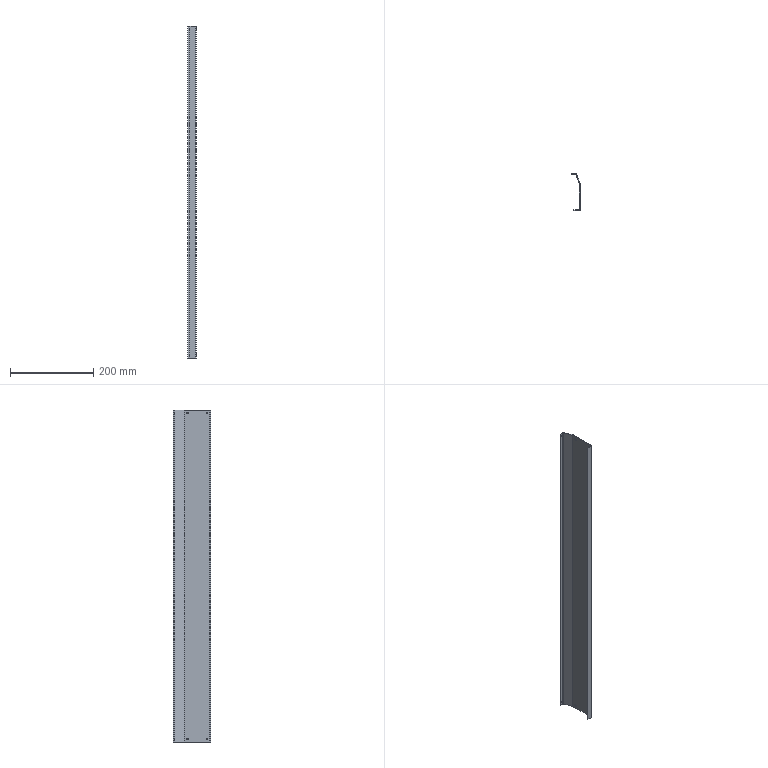Part | STEP file | In/out guide rail cover plate 2 | 1 solid | 41 faces | box 20 x 90 x 800 mm | volume 180213 mm3 | cylinder 17 | cone 12 | plane 12 | commonest cylinder face diameters 3.5 x12 4 x5
STEP:
#1=CARTESIAN_POINT('',(296.,43.65,-394.25));
#2=VERTEX_POINT('',#1);
#3=CARTESIAN_POINT('',(296.,43.65,-390.75));
#4=VERTEX_POINT('',#3);
#5=CARTESIAN_POINT('',(296.,43.65,-392.5));
#6=DIRECTION('',(0.,1.,0.));
#7=DIRECTION('',(0.,0.,1.));
#8=AXIS2_PLACEMENT_3D('',#5,#6,#7);
#9=CIRCLE('',#8,1.75);
#10=EDGE_CURVE('',#2,#4,#9,.T.);
#11=ORIENTED_EDGE('',*,*,#10,.F.);
#12=CARTESIAN_POINT('',(296.,45.,-395.6));
#13=VERTEX_POINT('',#12);
#14=CARTESIAN_POINT('',(296.,45.,-395.6));
#15=DIRECTION('',(0.,0.7071,-0.7071));
#16=VECTOR('',#15,1000.);
#17=LINE('',#14,#16);
#18=EDGE_CURVE('',#2,#13,#17,.T.);
#19=ORIENTED_EDGE('',*,*,#18,.T.);
#20=CARTESIAN_POINT('',(296.,45.,-389.4));
#21=VERTEX_POINT('',#20);
#22=CARTESIAN_POINT('',(296.,45.,-392.5));
#23=DIRECTION('',(0.,1.,0.));
#24=DIRECTION('',(0.,0.,1.));
#25=AXIS2_PLACEMENT_3D('',#22,#23,#24);
#26=CIRCLE('',#25,3.1);
#27=EDGE_CURVE('',#13,#21,#26,.T.);
#28=ORIENTED_EDGE('',*,*,#27,.T.);
#29=CARTESIAN_POINT('',(296.,45.,-389.4));
#30=DIRECTION('',(0.,0.7071,0.7071));
#31=VECTOR('',#30,1000.);
#32=LINE('',#29,#31);
#33=EDGE_CURVE('',#4,#21,#32,.T.);
#34=ORIENTED_EDGE('',*,*,#33,.F.);
#35=EDGE_LOOP('',(#11,#19,#28,#34));
#36=FACE_OUTER_BOUND('',#35,.T.);
#37=CARTESIAN_POINT('',(296.,45.,-392.5));
#38=DIRECTION('',(0.,1.,0.));
#39=DIRECTION('',(0.,0.,1.));
#40=AXIS2_PLACEMENT_3D('',#37,#38,#39);
#41=CONICAL_SURFACE('',#40,3.1,0.7854);
#42=ADVANCED_FACE('',(#36),#41,.F.);
#43=CARTESIAN_POINT('',(296.,43.,-394.25));
#44=VERTEX_POINT('',#43);
#45=CARTESIAN_POINT('',(296.,43.,-390.75));
#46=VERTEX_POINT('',#45);
#47=CARTESIAN_POINT('',(296.,43.,-392.5));
#48=DIRECTION('',(0.,1.,0.));
#49=DIRECTION('',(-1.,0.,0.));
#50=AXIS2_PLACEMENT_3D('',#47,#48,#49);
#51=CIRCLE('',#50,1.75);
#52=EDGE_CURVE('',#44,#46,#51,.T.);
#53=ORIENTED_EDGE('',*,*,#52,.F.);
#54=CARTESIAN_POINT('',(296.,45.,-394.25));
#55=DIRECTION('',(0.,1.,0.));
#56=VECTOR('',#55,1000.);
#57=LINE('',#54,#56);
#58=EDGE_CURVE('',#44,#2,#57,.T.);
#59=ORIENTED_EDGE('',*,*,#58,.T.);
#60=ORIENTED_EDGE('',*,*,#10,.T.);
#61=CARTESIAN_POINT('',(296.,45.,-390.75));
#62=DIRECTION('',(0.,1.,0.));
#63=VECTOR('',#62,1000.);
#64=LINE('',#61,#63);
#65=EDGE_CURVE('',#46,#4,#64,.T.);
#66=ORIENTED_EDGE('',*,*,#65,.F.);
#67=EDGE_LOOP('',(#53,#59,#60,#66));
#68=FACE_OUTER_BOUND('',#67,.T.);
#69=CARTESIAN_POINT('',(296.,45.,-392.5));
#70=DIRECTION('',(0.,1.,0.));
#71=DIRECTION('',(0.,0.,1.));
#72=AXIS2_PLACEMENT_3D('',#69,#70,#71);
#73=CYLINDRICAL_SURFACE('',#72,1.75);
#74=ADVANCED_FACE('',(#68),#73,.F.);
#75=CARTESIAN_POINT('',(296.,43.65,390.75));
#76=VERTEX_POINT('',#75);
#77=CARTESIAN_POINT('',(296.,43.65,394.25));
#78=VERTEX_POINT('',#77);
#79=CARTESIAN_POINT('',(296.,43.65,392.5));
#80=DIRECTION('',(0.,1.,0.));
#81=DIRECTION('',(0.,0.,1.));
#82=AXIS2_PLACEMENT_3D('',#79,#80,#81);
#83=CIRCLE('',#82,1.75);
#84=EDGE_CURVE('',#76,#78,#83,.T.);
#85=ORIENTED_EDGE('',*,*,#84,.F.);
#86=CARTESIAN_POINT('',(296.,45.,389.4));
#87=VERTEX_POINT('',#86);
#88=CARTESIAN_POINT('',(296.,45.,389.4));
#89=DIRECTION('',(0.,0.7071,-0.7071));
#90=VECTOR('',#89,1000.);
#91=LINE('',#88,#90);
#92=EDGE_CURVE('',#76,#87,#91,.T.);
#93=ORIENTED_EDGE('',*,*,#92,.T.);
#94=CARTESIAN_POINT('',(296.,45.,395.6));
#95=VERTEX_POINT('',#94);
#96=CARTESIAN_POINT('',(296.,45.,392.5));
#97=DIRECTION('',(0.,1.,0.));
#98=DIRECTION('',(0.,0.,1.));
#99=AXIS2_PLACEMENT_3D('',#96,#97,#98);
#100=CIRCLE('',#99,3.1);
#101=EDGE_CURVE('',#87,#95,#100,.T.);
#102=ORIENTED_EDGE('',*,*,#101,.T.);
#103=CARTESIAN_POINT('',(296.,45.,395.6));
#104=DIRECTION('',(0.,0.7071,0.7071));
#105=VECTOR('',#104,1000.);
#106=LINE('',#103,#105);
#107=EDGE_CURVE('',#78,#95,#106,.T.);
#108=ORIENTED_EDGE('',*,*,#107,.F.);
#109=EDGE_LOOP('',(#85,#93,#102,#108));
#110=FACE_OUTER_BOUND('',#109,.T.);
#111=CARTESIAN_POINT('',(296.,45.,392.5));
#112=DIRECTION('',(0.,1.,0.));
#113=DIRECTION('',(0.,0.,1.));
#114=AXIS2_PLACEMENT_3D('',#111,#112,#113);
#115=CONICAL_SURFACE('',#114,3.1,0.7854);
#116=ADVANCED_FACE('',(#110),#115,.F.);
#117=CARTESIAN_POINT('',(296.,43.,390.75));
#118=VERTEX_POINT('',#117);
#119=CARTESIAN_POINT('',(296.,43.,394.25));
#120=VERTEX_POINT('',#119);
#121=CARTESIAN_POINT('',(296.,43.,392.5));
#122=DIRECTION('',(0.,1.,0.));
#123=DIRECTION('',(-1.,0.,0.));
#124=AXIS2_PLACEMENT_3D('',#121,#122,#123);
#125=CIRCLE('',#124,1.75);
#126=EDGE_CURVE('',#118,#120,#125,.T.);
#127=ORIENTED_EDGE('',*,*,#126,.F.);
#128=CARTESIAN_POINT('',(296.,45.,390.75));
#129=DIRECTION('',(0.,1.,0.));
#130=VECTOR('',#129,1000.);
#131=LINE('',#128,#130);
#132=EDGE_CURVE('',#118,#76,#131,.T.);
#133=ORIENTED_EDGE('',*,*,#132,.T.);
#134=ORIENTED_EDGE('',*,*,#84,.T.);
#135=CARTESIAN_POINT('',(296.,45.,394.25));
#136=DIRECTION('',(0.,1.,0.));
#137=VECTOR('',#136,1000.);
#138=LINE('',#135,#137);
#139=EDGE_CURVE('',#120,#78,#138,.T.);
#140=ORIENTED_EDGE('',*,*,#139,.F.);
#141=EDGE_LOOP('',(#127,#133,#134,#140));
#142=FACE_OUTER_BOUND('',#141,.T.);
#143=CARTESIAN_POINT('',(296.,45.,392.5));
#144=DIRECTION('',(0.,1.,0.));
#145=DIRECTION('',(0.,0.,1.));
#146=AXIS2_PLACEMENT_3D('',#143,#144,#145);
#147=CYLINDRICAL_SURFACE('',#146,1.75);
#148=ADVANCED_FACE('',(#142),#147,.F.);
#149=CARTESIAN_POINT('',(309.447,10.5,-390.75));
#150=VERTEX_POINT('',#149);
#151=CARTESIAN_POINT('',(309.447,10.5,-394.25));
#152=VERTEX_POINT('',#151);
#153=CARTESIAN_POINT('',(309.447,10.5,-392.5));
#154=DIRECTION('',(1.,0.,0.));
#155=DIRECTION('',(0.,0.,-1.));
#156=AXIS2_PLACEMENT_3D('',#153,#154,#155);
#157=CIRCLE('',#156,1.75);
#158=EDGE_CURVE('',#150,#152,#157,.T.);
#159=ORIENTED_EDGE('',*,*,#158,.F.);
#160=CARTESIAN_POINT('',(311.,10.5,-389.4));
#161=VERTEX_POINT('',#160);
#162=CARTESIAN_POINT('',(311.,10.5,-389.4));
#163=DIRECTION('',(0.7547,0.,0.6561));
#164=VECTOR('',#163,1000.);
#165=LINE('',#162,#164);
#166=EDGE_CURVE('',#150,#161,#165,.T.);
#167=ORIENTED_EDGE('',*,*,#166,.T.);
#168=CARTESIAN_POINT('',(311.,10.5,-395.6));
#169=VERTEX_POINT('',#168);
#170=CARTESIAN_POINT('',(311.,10.5,-392.5));
#171=DIRECTION('',(1.,0.,0.));
#172=DIRECTION('',(0.,0.,-1.));
#173=AXIS2_PLACEMENT_3D('',#170,#171,#172);
#174=CIRCLE('',#173,3.1);
#175=EDGE_CURVE('',#161,#169,#174,.T.);
#176=ORIENTED_EDGE('',*,*,#175,.T.);
#177=CARTESIAN_POINT('',(311.,10.5,-395.6));
#178=DIRECTION('',(0.7547,0.,-0.6561));
#179=VECTOR('',#178,1000.);
#180=LINE('',#177,#179);
#181=EDGE_CURVE('',#152,#169,#180,.T.);
#182=ORIENTED_EDGE('',*,*,#181,.F.);
#183=EDGE_LOOP('',(#159,#167,#176,#182));
#184=FACE_OUTER_BOUND('',#183,.T.);
#185=CARTESIAN_POINT('',(311.,10.5,-392.5));
#186=DIRECTION('',(1.,0.,0.));
#187=DIRECTION('',(0.,0.,-1.));
#188=AXIS2_PLACEMENT_3D('',#185,#186,#187);
#189=CONICAL_SURFACE('',#188,3.1,0.7156);
#190=ADVANCED_FACE('',(#184),#189,.F.);
#191=CARTESIAN_POINT('',(309.,10.5,-390.75));
#192=VERTEX_POINT('',#191);
#193=CARTESIAN_POINT('',(309.,10.5,-394.25));
#194=VERTEX_POINT('',#193);
#195=CARTESIAN_POINT('',(309.,10.5,-392.5));
#196=DIRECTION('',(1.,0.,0.));
#197=DIRECTION('',(0.,0.,-1.));
#198=AXIS2_PLACEMENT_3D('',#195,#196,#197);
#199=CIRCLE('',#198,1.75);
#200=EDGE_CURVE('',#192,#194,#199,.T.);
#201=ORIENTED_EDGE('',*,*,#200,.F.);
#202=CARTESIAN_POINT('',(311.,10.5,-390.75));
#203=DIRECTION('',(1.,0.,0.));
#204=VECTOR('',#203,1000.);
#205=LINE('',#202,#204);
#206=EDGE_CURVE('',#192,#150,#205,.T.);
#207=ORIENTED_EDGE('',*,*,#206,.T.);
#208=ORIENTED_EDGE('',*,*,#158,.T.);
#209=CARTESIAN_POINT('',(311.,10.5,-394.25));
#210=DIRECTION('',(1.,0.,0.));
#211=VECTOR('',#210,1000.);
#212=LINE('',#209,#211);
#213=EDGE_CURVE('',#194,#152,#212,.T.);
#214=ORIENTED_EDGE('',*,*,#213,.F.);
#215=EDGE_LOOP('',(#201,#207,#208,#214));
#216=FACE_OUTER_BOUND('',#215,.T.);
#217=CARTESIAN_POINT('',(311.,10.5,-392.5));
#218=DIRECTION('',(1.,0.,0.));
#219=DIRECTION('',(0.,0.,-1.));
#220=AXIS2_PLACEMENT_3D('',#217,#218,#219);
#221=CYLINDRICAL_SURFACE('',#220,1.75);
#222=ADVANCED_FACE('',(#216),#221,.F.);
#223=CARTESIAN_POINT('',(309.447,-35.5,394.25));
#224=VERTEX_POINT('',#223);
#225=CARTESIAN_POINT('',(309.447,-35.5,390.75));
#226=VERTEX_POINT('',#225);
#227=CARTESIAN_POINT('',(309.447,-35.5,392.5));
#228=DIRECTION('',(1.,0.,0.));
#229=DIRECTION('',(0.,0.,-1.));
#230=AXIS2_PLACEMENT_3D('',#227,#228,#229);
#231=CIRCLE('',#230,1.75);
#232=EDGE_CURVE('',#224,#226,#231,.T.);
#233=ORIENTED_EDGE('',*,*,#232,.F.);
#234=CARTESIAN_POINT('',(311.,-35.5,395.6));
#235=VERTEX_POINT('',#234);
#236=CARTESIAN_POINT('',(311.,-35.5,395.6));
#237=DIRECTION('',(0.7547,0.,0.6561));
#238=VECTOR('',#237,1000.);
#239=LINE('',#236,#238);
#240=EDGE_CURVE('',#224,#235,#239,.T.);
#241=ORIENTED_EDGE('',*,*,#240,.T.);
#242=CARTESIAN_POINT('',(311.,-35.5,389.4));
#243=VERTEX_POINT('',#242);
#244=CARTESIAN_POINT('',(311.,-35.5,392.5));
#245=DIRECTION('',(1.,0.,0.));
#246=DIRECTION('',(0.,0.,-1.));
#247=AXIS2_PLACEMENT_3D('',#244,#245,#246);
#248=CIRCLE('',#247,3.1);
#249=EDGE_CURVE('',#235,#243,#248,.T.);
#250=ORIENTED_EDGE('',*,*,#249,.T.);
#251=CARTESIAN_POINT('',(311.,-35.5,389.4));
#252=DIRECTION('',(0.7547,0.,-0.6561));
#253=VECTOR('',#252,1000.);
#254=LINE('',#251,#253);
#255=EDGE_CURVE('',#226,#243,#254,.T.);
#256=ORIENTED_EDGE('',*,*,#255,.F.);
#257=EDGE_LOOP('',(#233,#241,#250,#256));
#258=FACE_OUTER_BOUND('',#257,.T.);
#259=CARTESIAN_POINT('',(311.,-35.5,392.5));
#260=DIRECTION('',(1.,0.,0.));
#261=DIRECTION('',(0.,0.,-1.));
#262=AXIS2_PLACEMENT_3D('',#259,#260,#261);
#263=CONICAL_SURFACE('',#262,3.1,0.7156);
#264=ADVANCED_FACE('',(#258),#263,.F.);
#265=CARTESIAN_POINT('',(309.,-35.5,394.25));
#266=VERTEX_POINT('',#265);
#267=CARTESIAN_POINT('',(309.,-35.5,390.75));
#268=VERTEX_POINT('',#267);
#269=CARTESIAN_POINT('',(309.,-35.5,392.5));
#270=DIRECTION('',(1.,0.,0.));
#271=DIRECTION('',(0.,0.,-1.));
#272=AXIS2_PLACEMENT_3D('',#269,#270,#271);
#273=CIRCLE('',#272,1.75);
#274=EDGE_CURVE('',#266,#268,#273,.T.);
#275=ORIENTED_EDGE('',*,*,#274,.F.);
#276=CARTESIAN_POINT('',(311.,-35.5,394.25));
#277=DIRECTION('',(1.,0.,0.));
#278=VECTOR('',#277,1000.);
#279=LINE('',#276,#278);
#280=EDGE_CURVE('',#266,#224,#279,.T.);
#281=ORIENTED_EDGE('',*,*,#280,.T.);
#282=ORIENTED_EDGE('',*,*,#232,.T.);
#283=CARTESIAN_POINT('',(311.,-35.5,390.75));
#284=DIRECTION('',(1.,0.,0.));
#285=VECTOR('',#284,1000.);
#286=LINE('',#283,#285);
#287=EDGE_CURVE('',#268,#226,#286,.T.);
#288=ORIENTED_EDGE('',*,*,#287,.F.);
#289=EDGE_LOOP('',(#275,#281,#282,#288));
#290=FACE_OUTER_BOUND('',#289,.T.);
#291=CARTESIAN_POINT('',(311.,-35.5,392.5));
#292=DIRECTION('',(1.,0.,0.));
#293=DIRECTION('',(0.,0.,-1.));
#294=AXIS2_PLACEMENT_3D('',#291,#292,#293);
#295=CYLINDRICAL_SURFACE('',#294,1.75);
#296=ADVANCED_FACE('',(#290),#295,.F.);
#297=CARTESIAN_POINT('',(309.447,10.5,394.25));
#298=VERTEX_POINT('',#297);
#299=CARTESIAN_POINT('',(309.447,10.5,390.75));
#300=VERTEX_POINT('',#299);
#301=CARTESIAN_POINT('',(309.447,10.5,392.5));
#302=DIRECTION('',(1.,0.,0.));
#303=DIRECTION('',(0.,0.,-1.));
#304=AXIS2_PLACEMENT_3D('',#301,#302,#303);
#305=CIRCLE('',#304,1.75);
#306=EDGE_CURVE('',#298,#300,#305,.T.);
#307=ORIENTED_EDGE('',*,*,#306,.F.);
#308=CARTESIAN_POINT('',(311.,10.5,395.6));
#309=VERTEX_POINT('',#308);
#310=CARTESIAN_POINT('',(311.,10.5,395.6));
#311=DIRECTION('',(0.7547,0.,0.6561));
#312=VECTOR('',#311,1000.);
#313=LINE('',#310,#312);
#314=EDGE_CURVE('',#298,#309,#313,.T.);
#315=ORIENTED_EDGE('',*,*,#314,.T.);
#316=CARTESIAN_POINT('',(311.,10.5,389.4));
#317=VERTEX_POINT('',#316);
#318=CARTESIAN_POINT('',(311.,10.5,392.5));
#319=DIRECTION('',(1.,0.,0.));
#320=DIRECTION('',(0.,0.,-1.));
#321=AXIS2_PLACEMENT_3D('',#318,#319,#320);
#322=CIRCLE('',#321,3.1);
#323=EDGE_CURVE('',#309,#317,#322,.T.);
#324=ORIENTED_EDGE('',*,*,#323,.T.);
#325=CARTESIAN_POINT('',(311.,10.5,389.4));
#326=DIRECTION('',(0.7547,0.,-0.6561));
#327=VECTOR('',#326,1000.);
#328=LINE('',#325,#327);
#329=EDGE_CURVE('',#300,#317,#328,.T.);
#330=ORIENTED_EDGE('',*,*,#329,.F.);
#331=EDGE_LOOP('',(#307,#315,#324,#330));
#332=FACE_OUTER_BOUND('',#331,.T.);
#333=CARTESIAN_POINT('',(311.,10.5,392.5));
#334=DIRECTION('',(1.,0.,0.));
#335=DIRECTION('',(0.,0.,-1.));
#336=AXIS2_PLACEMENT_3D('',#333,#334,#335);
#337=CONICAL_SURFACE('',#336,3.1,0.7156);
#338=ADVANCED_FACE('',(#332),#337,.F.);
#339=CARTESIAN_POINT('',(309.,10.5,394.25));
#340=VERTEX_POINT('',#339);
#341=CARTESIAN_POINT('',(309.,10.5,390.75));
#342=VERTEX_POINT('',#341);
#343=CARTESIAN_POINT('',(309.,10.5,392.5));
#344=DIRECTION('',(1.,0.,0.));
#345=DIRECTION('',(0.,0.,-1.));
#346=AXIS2_PLACEMENT_3D('',#343,#344,#345);
#347=CIRCLE('',#346,1.75);
#348=EDGE_CURVE('',#340,#342,#347,.T.);
#349=ORIENTED_EDGE('',*,*,#348,.F.);
#350=CARTESIAN_POINT('',(311.,10.5,394.25));
#351=DIRECTION('',(1.,0.,0.));
#352=VECTOR('',#351,1000.);
#353=LINE('',#350,#352);
#354=EDGE_CURVE('',#340,#298,#353,.T.);
#355=ORIENTED_EDGE('',*,*,#354,.T.);
#356=ORIENTED_EDGE('',*,*,#306,.T.);
#357=CARTESIAN_POINT('',(311.,10.5,390.75));
#358=DIRECTION('',(1.,0.,0.));
#359=VECTOR('',#358,1000.);
#360=LINE('',#357,#359);
#361=EDGE_CURVE('',#342,#300,#360,.T.);
#362=ORIENTED_EDGE('',*,*,#361,.F.);
#363=EDGE_LOOP('',(#349,#355,#356,#362));
#364=FACE_OUTER_BOUND('',#363,.T.);
#365=CARTESIAN_POINT('',(311.,10.5,392.5));
#366=DIRECTION('',(1.,0.,0.));
#367=DIRECTION('',(0.,0.,-1.));
#368=AXIS2_PLACEMENT_3D('',#365,#366,#367);
#369=CYLINDRICAL_SURFACE('',#368,1.75);
#370=ADVANCED_FACE('',(#364),#369,.F.);
#371=CARTESIAN_POINT('',(309.447,-35.5,-390.75));
#372=VERTEX_POINT('',#371);
#373=CARTESIAN_POINT('',(309.447,-35.5,-394.25));
#374=VERTEX_POINT('',#373);
#375=CARTESIAN_POINT('',(309.447,-35.5,-392.5));
#376=DIRECTION('',(1.,0.,0.));
#377=DIRECTION('',(0.,0.,-1.));
#378=AXIS2_PLACEMENT_3D('',#375,#376,#377);
#379=CIRCLE('',#378,1.75);
#380=EDGE_CURVE('',#372,#374,#379,.T.);
#381=ORIENTED_EDGE('',*,*,#380,.F.);
#382=CARTESIAN_POINT('',(311.,-35.5,-389.4));
#383=VERTEX_POINT('',#382);
#384=CARTESIAN_POINT('',(311.,-35.5,-389.4));
#385=DIRECTION('',(0.7547,0.,0.6561));
#386=VECTOR('',#385,1000.);
#387=LINE('',#384,#386);
#388=EDGE_CURVE('',#372,#383,#387,.T.);
#389=ORIENTED_EDGE('',*,*,#388,.T.);
#390=CARTESIAN_POINT('',(311.,-35.5,-395.6));
#391=VERTEX_POINT('',#390);
#392=CARTESIAN_POINT('',(311.,-35.5,-392.5));
#393=DIRECTION('',(1.,0.,0.));
#394=DIRECTION('',(0.,0.,-1.));
#395=AXIS2_PLACEMENT_3D('',#392,#393,#394);
#396=CIRCLE('',#395,3.1);
#397=EDGE_CURVE('',#383,#391,#396,.T.);
#398=ORIENTED_EDGE('',*,*,#397,.T.);
#399=CARTESIAN_POINT('',(311.,-35.5,-395.6));
#400=DIRECTION('',(0.7547,0.,-0.6561));
#401=VECTOR('',#400,1000.);
#402=LINE('',#399,#401);
#403=EDGE_CURVE('',#374,#391,#402,.T.);
#404=ORIENTED_EDGE('',*,*,#403,.F.);
#405=EDGE_LOOP('',(#381,#389,#398,#404));
#406=FACE_OUTER_BOUND('',#405,.T.);
#407=CARTESIAN_POINT('',(311.,-35.5,-392.5));
#408=DIRECTION('',(1.,0.,0.));
#409=DIRECTION('',(0.,0.,-1.));
#410=AXIS2_PLACEMENT_3D('',#407,#408,#409);
#411=CONICAL_SURFACE('',#410,3.1,0.7156);
#412=ADVANCED_FACE('',(#406),#411,.F.);
#413=CARTESIAN_POINT('',(309.,-35.5,-390.75));
#414=VERTEX_POINT('',#413);
#415=CARTESIAN_POINT('',(309.,-35.5,-394.25));
#416=VERTEX_POINT('',#415);
#417=CARTESIAN_POINT('',(309.,-35.5,-392.5));
#418=DIRECTION('',(1.,0.,0.));
#419=DIRECTION('',(0.,0.,-1.));
#420=AXIS2_PLACEMENT_3D('',#417,#418,#419);
#421=CIRCLE('',#420,1.75);
#422=EDGE_CURVE('',#414,#416,#421,.T.);
#423=ORIENTED_EDGE('',*,*,#422,.F.);
#424=CARTESIAN_POINT('',(311.,-35.5,-390.75));
#425=DIRECTION('',(1.,0.,0.));
#426=VECTOR('',#425,1000.);
#427=LINE('',#424,#426);
#428=EDGE_CURVE('',#414,#372,#427,.T.);
#429=ORIENTED_EDGE('',*,*,#428,.T.);
#430=ORIENTED_EDGE('',*,*,#380,.T.);
#431=CARTESIAN_POINT('',(311.,-35.5,-394.25));
#432=DIRECTION('',(1.,0.,0.));
#433=VECTOR('',#432,1000.);
#434=LINE('',#431,#433);
#435=EDGE_CURVE('',#416,#374,#434,.T.);
#436=ORIENTED_EDGE('',*,*,#435,.F.);
#437=EDGE_LOOP('',(#423,#429,#430,#436));
#438=FACE_OUTER_BOUND('',#437,.T.);
#439=CARTESIAN_POINT('',(311.,-35.5,-392.5));
#440=DIRECTION('',(1.,0.,0.));
#441=DIRECTION('',(0.,0.,-1.));
#442=AXIS2_PLACEMENT_3D('',#439,#440,#441);
#443=CYLINDRICAL_SURFACE('',#442,1.75);
#444=ADVANCED_FACE('',(#438),#443,.F.);
#445=CARTESIAN_POINT('',(309.,10.5,-392.5));
#446=DIRECTION('',(1.,0.,0.));
#447=DIRECTION('',(0.,0.,-1.));
#448=AXIS2_PLACEMENT_3D('',#445,#446,#447);
#449=CIRCLE('',#448,1.75);
#450=EDGE_CURVE('',#194,#192,#449,.T.);
#451=ORIENTED_EDGE('',*,*,#450,.T.);
#452=ORIENTED_EDGE('',*,*,#200,.T.);
#453=EDGE_LOOP('',(#451,#452));
#454=FACE_BOUND('',#453,.T.);
#455=CARTESIAN_POINT('',(309.,-35.5,392.5));
#456=DIRECTION('',(1.,0.,0.));
#457=DIRECTION('',(0.,0.,-1.));
#458=AXIS2_PLACEMENT_3D('',#455,#456,#457);
#459=CIRCLE('',#458,1.75);
#460=EDGE_CURVE('',#268,#266,#459,.T.);
#461=ORIENTED_EDGE('',*,*,#460,.T.);
#462=ORIENTED_EDGE('',*,*,#274,.T.);
#463=EDGE_LOOP('',(#461,#462));
#464=FACE_BOUND('',#463,.T.);
#465=CARTESIAN_POINT('',(309.,10.5,392.5));
#466=DIRECTION('',(1.,0.,0.));
#467=DIRECTION('',(0.,0.,-1.));
#468=AXIS2_PLACEMENT_3D('',#465,#466,#467);
#469=CIRCLE('',#468,1.75);
#470=EDGE_CURVE('',#342,#340,#469,.T.);
#471=ORIENTED_EDGE('',*,*,#470,.T.);
#472=ORIENTED_EDGE('',*,*,#348,.T.);
#473=EDGE_LOOP('',(#471,#472));
#474=FACE_BOUND('',#473,.T.);
#475=CARTESIAN_POINT('',(309.,-35.5,-392.5));
#476=DIRECTION('',(1.,0.,0.));
#477=DIRECTION('',(0.,0.,-1.));
#478=AXIS2_PLACEMENT_3D('',#475,#476,#477);
#479=CIRCLE('',#478,1.75);
#480=EDGE_CURVE('',#416,#414,#479,.T.);
#481=ORIENTED_EDGE('',*,*,#480,.T.);
#482=ORIENTED_EDGE('',*,*,#422,.T.);
#483=EDGE_LOOP('',(#481,#482));
#484=FACE_BOUND('',#483,.T.);
#485=CARTESIAN_POINT('',(309.,19.23,400.));
#486=VERTEX_POINT('',#485);
#487=CARTESIAN_POINT('',(309.,-43.,400.));
#488=VERTEX_POINT('',#487);
#489=CARTESIAN_POINT('',(309.,19.615,400.));
#490=DIRECTION('',(0.,-1.,0.));
#491=VECTOR('',#490,1000.);
#492=LINE('',#489,#491);
#493=EDGE_CURVE('',#486,#488,#492,.T.);
#494=ORIENTED_EDGE('',*,*,#493,.F.);
#495=CARTESIAN_POINT('',(309.,19.23,-400.));
#496=VERTEX_POINT('',#495);
#497=CARTESIAN_POINT('',(309.,19.23,-400.));
#498=DIRECTION('',(0.,0.,-1.));
#499=VECTOR('',#498,1000.);
#500=LINE('',#497,#499);
#501=EDGE_CURVE('',#486,#496,#500,.T.);
#502=ORIENTED_EDGE('',*,*,#501,.T.);
#503=CARTESIAN_POINT('',(309.,-43.,-400.));
#504=VERTEX_POINT('',#503);
#505=CARTESIAN_POINT('',(309.,19.615,-400.));
#506=DIRECTION('',(0.,-1.,0.));
#507=VECTOR('',#506,1000.);
#508=LINE('',#505,#507);
#509=EDGE_CURVE('',#496,#504,#508,.T.);
#510=ORIENTED_EDGE('',*,*,#509,.T.);
#511=CARTESIAN_POINT('',(309.,-43.,-400.));
#512=DIRECTION('',(0.,0.,-1.));
#513=VECTOR('',#512,1000.);
#514=LINE('',#511,#513);
#515=EDGE_CURVE('',#488,#504,#514,.T.);
#516=ORIENTED_EDGE('',*,*,#515,.F.);
#517=EDGE_LOOP('',(#494,#502,#510,#516));
#518=FACE_OUTER_BOUND('',#517,.T.);
#519=CARTESIAN_POINT('',(309.,19.615,400.));
#520=DIRECTION('',(1.,0.,0.));
#521=DIRECTION('',(0.,0.,-1.));
#522=AXIS2_PLACEMENT_3D('',#519,#520,#521);
#523=PLANE('',#522);
#524=ADVANCED_FACE('',(#454,#464,#474,#484,#518),#523,.F.);
#525=CARTESIAN_POINT('',(296.,45.,-392.5));
#526=DIRECTION('',(0.,1.,0.));
#527=DIRECTION('',(0.,0.,1.));
#528=AXIS2_PLACEMENT_3D('',#525,#526,#527);
#529=CIRCLE('',#528,3.1);
#530=EDGE_CURVE('',#21,#13,#529,.T.);
#531=ORIENTED_EDGE('',*,*,#530,.F.);
#532=ORIENTED_EDGE('',*,*,#27,.F.);
#533=EDGE_LOOP('',(#531,#532));
#534=FACE_BOUND('',#533,.T.);
#535=CARTESIAN_POINT('',(296.,45.,392.5));
#536=DIRECTION('',(0.,1.,0.));
#537=DIRECTION('',(0.,0.,1.));
#538=AXIS2_PLACEMENT_3D('',#535,#536,#537);
#539=CIRCLE('',#538,3.1);
#540=EDGE_CURVE('',#95,#87,#539,.T.);
#541=ORIENTED_EDGE('',*,*,#540,.F.);
#542=ORIENTED_EDGE('',*,*,#101,.F.);
#543=EDGE_LOOP('',(#541,#542));
#544=FACE_BOUND('',#543,.T.);
#545=CARTESIAN_POINT('',(299.646,45.,400.));
#546=VERTEX_POINT('',#545);
#547=CARTESIAN_POINT('',(291.,45.,400.));
#548=VERTEX_POINT('',#547);
#549=CARTESIAN_POINT('',(301.,45.,400.));
#550=DIRECTION('',(-1.,0.,0.));
#551=VECTOR('',#550,1000.);
#552=LINE('',#549,#551);
#553=EDGE_CURVE('',#546,#548,#552,.T.);
#554=ORIENTED_EDGE('',*,*,#553,.F.);
#555=CARTESIAN_POINT('',(299.646,45.,-400.));
#556=VERTEX_POINT('',#555);
#557=CARTESIAN_POINT('',(299.646,45.,-400.));
#558=DIRECTION('',(0.,0.,-1.));
#559=VECTOR('',#558,1000.);
#560=LINE('',#557,#559);
#561=EDGE_CURVE('',#546,#556,#560,.T.);
#562=ORIENTED_EDGE('',*,*,#561,.T.);
#563=CARTESIAN_POINT('',(291.,45.,-400.));
#564=VERTEX_POINT('',#563);
#565=CARTESIAN_POINT('',(301.,45.,-400.));
#566=DIRECTION('',(-1.,0.,0.));
#567=VECTOR('',#566,1000.);
#568=LINE('',#565,#567);
#569=EDGE_CURVE('',#556,#564,#568,.T.);
#570=ORIENTED_EDGE('',*,*,#569,.T.);
#571=CARTESIAN_POINT('',(291.,45.,-400.));
#572=DIRECTION('',(0.,0.,1.));
#573=VECTOR('',#572,1000.);
#574=LINE('',#571,#573);
#575=EDGE_CURVE('',#564,#548,#574,.T.);
#576=ORIENTED_EDGE('',*,*,#575,.T.);
#577=EDGE_LOOP('',(#554,#562,#570,#576));
#578=FACE_OUTER_BOUND('',#577,.T.);
#579=CARTESIAN_POINT('',(301.,45.,-400.));
#580=DIRECTION('',(0.,1.,0.));
#581=DIRECTION('',(0.,0.,1.));
#582=AXIS2_PLACEMENT_3D('',#579,#580,#581);
#583=PLANE('',#582);
#584=ADVANCED_FACE('',(#534,#544,#578),#583,.T.);
#585=CARTESIAN_POINT('',(310.857,20.358,400.));
#586=VERTEX_POINT('',#585);
#587=CARTESIAN_POINT('',(301.503,43.743,400.));
#588=VERTEX_POINT('',#587);
#589=CARTESIAN_POINT('',(311.,20.,400.));
#590=DIRECTION('',(-0.3714,0.9285,0.));
#591=VECTOR('',#590,1000.);
#592=LINE('',#589,#591);
#593=EDGE_CURVE('',#586,#588,#592,.T.);
#594=ORIENTED_EDGE('',*,*,#593,.F.);
#595=CARTESIAN_POINT('',(310.857,20.358,-400.));
#596=VERTEX_POINT('',#595);
#597=CARTESIAN_POINT('',(310.857,20.358,-400.));
#598=DIRECTION('',(0.,0.,-1.));
#599=VECTOR('',#598,1000.);
#600=LINE('',#597,#599);
#601=EDGE_CURVE('',#586,#596,#600,.T.);
#602=ORIENTED_EDGE('',*,*,#601,.T.);
#603=CARTESIAN_POINT('',(301.503,43.743,-400.));
#604=VERTEX_POINT('',#603);
#605=CARTESIAN_POINT('',(311.,20.,-400.));
#606=DIRECTION('',(-0.3714,0.9285,0.));
#607=VECTOR('',#606,1000.);
#608=LINE('',#605,#607);
#609=EDGE_CURVE('',#596,#604,#608,.T.);
#610=ORIENTED_EDGE('',*,*,#609,.T.);
#611=CARTESIAN_POINT('',(301.503,43.743,-400.));
#612=DIRECTION('',(0.,0.,1.));
#613=VECTOR('',#612,1000.);
#614=LINE('',#611,#613);
#615=EDGE_CURVE('',#604,#588,#614,.T.);
#616=ORIENTED_EDGE('',*,*,#615,.T.);
#617=EDGE_LOOP('',(#594,#602,#610,#616));
#618=FACE_OUTER_BOUND('',#617,.T.);
#619=CARTESIAN_POINT('',(311.,20.,-400.));
#620=DIRECTION('',(0.9285,0.3714,0.));
#621=DIRECTION('',(-0.3714,0.9285,0.));
#622=AXIS2_PLACEMENT_3D('',#619,#620,#621);
#623=PLANE('',#622);
#624=ADVANCED_FACE('',(#618),#623,.T.);
#625=CARTESIAN_POINT('',(311.,10.5,-392.5));
#626=DIRECTION('',(1.,0.,0.));
#627=DIRECTION('',(0.,0.,-1.));
#628=AXIS2_PLACEMENT_3D('',#625,#626,#627);
#629=CIRCLE('',#628,3.1);
#630=EDGE_CURVE('',#169,#161,#629,.T.);
#631=ORIENTED_EDGE('',*,*,#630,.F.);
#632=ORIENTED_EDGE('',*,*,#175,.F.);
#633=EDGE_LOOP('',(#631,#632));
#634=FACE_BOUND('',#633,.T.);
#635=CARTESIAN_POINT('',(311.,-35.5,392.5));
#636=DIRECTION('',(1.,0.,0.));
#637=DIRECTION('',(0.,0.,-1.));
#638=AXIS2_PLACEMENT_3D('',#635,#636,#637);
#639=CIRCLE('',#638,3.1);
#640=EDGE_CURVE('',#243,#235,#639,.T.);
#641=ORIENTED_EDGE('',*,*,#640,.F.);
#642=ORIENTED_EDGE('',*,*,#249,.F.);
#643=EDGE_LOOP('',(#641,#642));
#644=FACE_BOUND('',#643,.T.);
#645=CARTESIAN_POINT('',(311.,10.5,392.5));
#646=DIRECTION('',(1.,0.,0.));
#647=DIRECTION('',(0.,0.,-1.));
#648=AXIS2_PLACEMENT_3D('',#645,#646,#647);
#649=CIRCLE('',#648,3.1);
#650=EDGE_CURVE('',#317,#309,#649,.T.);
#651=ORIENTED_EDGE('',*,*,#650,.F.);
#652=ORIENTED_EDGE('',*,*,#323,.F.);
#653=EDGE_LOOP('',(#651,#652));
#654=FACE_BOUND('',#653,.T.);
#655=CARTESIAN_POINT('',(311.,-35.5,-392.5));
#656=DIRECTION('',(1.,0.,0.));
#657=DIRECTION('',(0.,0.,-1.));
#658=AXIS2_PLACEMENT_3D('',#655,#656,#657);
#659=CIRCLE('',#658,3.1);
#660=EDGE_CURVE('',#391,#383,#659,.T.);
#661=ORIENTED_EDGE('',*,*,#660,.F.);
#662=ORIENTED_EDGE('',*,*,#397,.F.);
#663=EDGE_LOOP('',(#661,#662));
#664=FACE_BOUND('',#663,.T.);
#665=CARTESIAN_POINT('',(311.,-43.,-400.));
#666=VERTEX_POINT('',#665);
#667=CARTESIAN_POINT('',(311.,19.615,-400.));
#668=VERTEX_POINT('',#667);
#669=CARTESIAN_POINT('',(311.,-45.,-400.));
#670=DIRECTION('',(0.,1.,0.));
#671=VECTOR('',#670,1000.);
#672=LINE('',#669,#671);
#673=EDGE_CURVE('',#666,#668,#672,.T.);
#674=ORIENTED_EDGE('',*,*,#673,.T.);
#675=CARTESIAN_POINT('',(311.,19.615,400.));
#676=VERTEX_POINT('',#675);
#677=CARTESIAN_POINT('',(311.,19.615,-400.));
#678=DIRECTION('',(0.,0.,1.));
#679=VECTOR('',#678,1000.);
#680=LINE('',#677,#679);
#681=EDGE_CURVE('',#668,#676,#680,.T.);
#682=ORIENTED_EDGE('',*,*,#681,.T.);
#683=CARTESIAN_POINT('',(311.,-43.,400.));
#684=VERTEX_POINT('',#683);
#685=CARTESIAN_POINT('',(311.,-45.,400.));
#686=DIRECTION('',(0.,1.,0.));
#687=VECTOR('',#686,1000.);
#688=LINE('',#685,#687);
#689=EDGE_CURVE('',#684,#676,#688,.T.);
#690=ORIENTED_EDGE('',*,*,#689,.F.);
#691=CARTESIAN_POINT('',(311.,-43.,-400.));
#692=DIRECTION('',(0.,0.,-1.));
#693=VECTOR('',#692,1000.);
#694=LINE('',#691,#693);
#695=EDGE_CURVE('',#684,#666,#694,.T.);
#696=ORIENTED_EDGE('',*,*,#695,.T.);
#697=EDGE_LOOP('',(#674,#682,#690,#696));
#698=FACE_OUTER_BOUND('',#697,.T.);
#699=CARTESIAN_POINT('',(311.,-45.,-400.));
#700=DIRECTION('',(1.,0.,0.));
#701=DIRECTION('',(0.,0.,-1.));
#702=AXIS2_PLACEMENT_3D('',#699,#700,#701);
#703=PLANE('',#702);
#704=ADVANCED_FACE('',(#634,#644,#654,#664,#698),#703,.T.);
#705=CARTESIAN_POINT('',(296.,-45.,-400.));
#706=VERTEX_POINT('',#705);
#707=CARTESIAN_POINT('',(309.,-45.,-400.));
#708=VERTEX_POINT('',#707);
#709=CARTESIAN_POINT('',(291.,-45.,-400.));
#710=DIRECTION('',(1.,0.,0.));
#711=VECTOR('',#710,1000.);
#712=LINE('',#709,#711);
#713=EDGE_CURVE('',#706,#708,#712,.T.);
#714=ORIENTED_EDGE('',*,*,#713,.T.);
#715=CARTESIAN_POINT('',(309.,-45.,400.));
#716=VERTEX_POINT('',#715);
#717=CARTESIAN_POINT('',(309.,-45.,-400.));
#718=DIRECTION('',(0.,0.,1.));
#719=VECTOR('',#718,1000.);
#720=LINE('',#717,#719);
#721=EDGE_CURVE('',#708,#716,#720,.T.);
#722=ORIENTED_EDGE('',*,*,#721,.T.);
#723=CARTESIAN_POINT('',(296.,-45.,400.));
#724=VERTEX_POINT('',#723);
#725=CARTESIAN_POINT('',(291.,-45.,400.));
#726=DIRECTION('',(1.,0.,0.));
#727=VECTOR('',#726,1000.);
#728=LINE('',#725,#727);
#729=EDGE_CURVE('',#724,#716,#728,.T.);
#730=ORIENTED_EDGE('',*,*,#729,.F.);
#731=CARTESIAN_POINT('',(296.,-45.,400.));
#732=DIRECTION('',(0.,0.,1.));
#733=VECTOR('',#732,1000.);
#734=LINE('',#731,#733);
#735=EDGE_CURVE('',#706,#724,#734,.T.);
#736=ORIENTED_EDGE('',*,*,#735,.F.);
#737=EDGE_LOOP('',(#714,#722,#730,#736));
#738=FACE_OUTER_BOUND('',#737,.T.);
#739=CARTESIAN_POINT('',(291.,-45.,-400.));
#740=DIRECTION('',(0.,-1.,0.));
#741=DIRECTION('',(0.,0.,-1.));
#742=AXIS2_PLACEMENT_3D('',#739,#740,#741);
#743=PLANE('',#742);
#744=ADVANCED_FACE('',(#738),#743,.T.);
#745=CARTESIAN_POINT('',(291.,43.,400.));
#746=VERTEX_POINT('',#745);
#747=CARTESIAN_POINT('',(291.,43.,-400.));
#748=VERTEX_POINT('',#747);
#749=CARTESIAN_POINT('',(291.,43.,400.));
#750=DIRECTION('',(0.,0.,-1.));
#751=VECTOR('',#750,1000.);
#752=LINE('',#749,#751);
#753=EDGE_CURVE('',#746,#748,#752,.T.);
#754=ORIENTED_EDGE('',*,*,#753,.F.);
#755=CARTESIAN_POINT('',(291.,45.,400.));
#756=DIRECTION('',(0.,-1.,0.));
#757=VECTOR('',#756,1000.);
#758=LINE('',#755,#757);
#759=EDGE_CURVE('',#548,#746,#758,.T.);
#760=ORIENTED_EDGE('',*,*,#759,.F.);
#761=ORIENTED_EDGE('',*,*,#575,.F.);
#762=CARTESIAN_POINT('',(291.,45.,-400.));
#763=DIRECTION('',(0.,-1.,0.));
#764=VECTOR('',#763,1000.);
#765=LINE('',#762,#764);
#766=EDGE_CURVE('',#564,#748,#765,.T.);
#767=ORIENTED_EDGE('',*,*,#766,.T.);
#768=EDGE_LOOP('',(#754,#760,#761,#767));
#769=FACE_OUTER_BOUND('',#768,.T.);
#770=CARTESIAN_POINT('',(291.,45.,-400.));
#771=DIRECTION('',(-1.,0.,0.));
#772=DIRECTION('',(0.,0.,1.));
#773=AXIS2_PLACEMENT_3D('',#770,#771,#772);
#774=PLANE('',#773);
#775=ADVANCED_FACE('',(#769),#774,.T.);
#776=ORIENTED_EDGE('',*,*,#609,.F.);
#777=CARTESIAN_POINT('',(309.,19.615,-400.));
#778=DIRECTION('',(0.,0.,-1.));
#779=DIRECTION('',(1.,0.,0.));
#780=AXIS2_PLACEMENT_3D('',#777,#778,#779);
#781=CIRCLE('',#780,2.);
#782=EDGE_CURVE('',#596,#668,#781,.T.);
#783=ORIENTED_EDGE('',*,*,#782,.T.);
#784=ORIENTED_EDGE('',*,*,#673,.F.);
#785=CARTESIAN_POINT('',(309.,-43.,-400.));
#786=DIRECTION('',(0.,0.,-1.));
#787=DIRECTION('',(1.,0.,0.));
#788=AXIS2_PLACEMENT_3D('',#785,#786,#787);
#789=CIRCLE('',#788,2.);
#790=EDGE_CURVE('',#666,#708,#789,.T.);
#791=ORIENTED_EDGE('',*,*,#790,.T.);
#792=ORIENTED_EDGE('',*,*,#713,.F.);
#793=CARTESIAN_POINT('',(296.,-43.,-400.));
#794=VERTEX_POINT('',#793);
#795=CARTESIAN_POINT('',(296.,-45.,-400.));
#796=DIRECTION('',(0.,-1.,0.));
#797=VECTOR('',#796,1000.);
#798=LINE('',#795,#797);
#799=EDGE_CURVE('',#794,#706,#798,.T.);
#800=ORIENTED_EDGE('',*,*,#799,.F.);
#801=CARTESIAN_POINT('',(296.,-43.,-400.));
#802=DIRECTION('',(1.,0.,0.));
#803=VECTOR('',#802,1000.);
#804=LINE('',#801,#803);
#805=EDGE_CURVE('',#794,#504,#804,.T.);
#806=ORIENTED_EDGE('',*,*,#805,.T.);
#807=ORIENTED_EDGE('',*,*,#509,.F.);
#808=CARTESIAN_POINT('',(308.857,19.972,-400.));
#809=VERTEX_POINT('',#808);
#810=CARTESIAN_POINT('',(307.,19.23,-400.));
#811=DIRECTION('',(0.,0.,1.));
#812=DIRECTION('',(1.,0.,0.));
#813=AXIS2_PLACEMENT_3D('',#810,#811,#812);
#814=CIRCLE('',#813,2.);
#815=EDGE_CURVE('',#496,#809,#814,.T.);
#816=ORIENTED_EDGE('',*,*,#815,.T.);
#817=CARTESIAN_POINT('',(300.149,41.743,-400.));
#818=VERTEX_POINT('',#817);
#819=CARTESIAN_POINT('',(299.646,43.,-400.));
#820=DIRECTION('',(0.3714,-0.9285,0.));
#821=VECTOR('',#820,1000.);
#822=LINE('',#819,#821);
#823=EDGE_CURVE('',#818,#809,#822,.T.);
#824=ORIENTED_EDGE('',*,*,#823,.F.);
#825=CARTESIAN_POINT('',(298.292,43.,-400.));
#826=VERTEX_POINT('',#825);
#827=CARTESIAN_POINT('',(298.292,41.,-400.));
#828=DIRECTION('',(0.,0.,1.));
#829=DIRECTION('',(1.,0.,0.));
#830=AXIS2_PLACEMENT_3D('',#827,#828,#829);
#831=CIRCLE('',#830,2.);
#832=EDGE_CURVE('',#818,#826,#831,.T.);
#833=ORIENTED_EDGE('',*,*,#832,.T.);
#834=CARTESIAN_POINT('',(291.,43.,-400.));
#835=DIRECTION('',(1.,0.,0.));
#836=VECTOR('',#835,1000.);
#837=LINE('',#834,#836);
#838=EDGE_CURVE('',#748,#826,#837,.T.);
#839=ORIENTED_EDGE('',*,*,#838,.F.);
#840=ORIENTED_EDGE('',*,*,#766,.F.);
#841=ORIENTED_EDGE('',*,*,#569,.F.);
#842=CARTESIAN_POINT('',(299.646,43.,-400.));
#843=DIRECTION('',(0.,0.,-1.));
#844=DIRECTION('',(1.,0.,0.));
#845=AXIS2_PLACEMENT_3D('',#842,#843,#844);
#846=CIRCLE('',#845,2.);
#847=EDGE_CURVE('',#556,#604,#846,.T.);
#848=ORIENTED_EDGE('',*,*,#847,.T.);
#849=EDGE_LOOP('',(#776,#783,#784,#791,#792,#800,#806,#807,#816,#824,#833,#839,#840,#841,#848));
#850=FACE_OUTER_BOUND('',#849,.T.);
#851=CARTESIAN_POINT('',(0.,0.,-400.));
#852=DIRECTION('',(0.,0.,1.));
#853=DIRECTION('',(1.,0.,0.));
#854=AXIS2_PLACEMENT_3D('',#851,#852,#853);
#855=PLANE('',#854);
#856=ADVANCED_FACE('',(#850),#855,.F.);
#857=ORIENTED_EDGE('',*,*,#689,.T.);
#858=CARTESIAN_POINT('',(309.,19.615,400.));
#859=DIRECTION('',(0.,0.,1.));
#860=DIRECTION('',(1.,0.,0.));
#861=AXIS2_PLACEMENT_3D('',#858,#859,#860);
#862=CIRCLE('',#861,2.);
#863=EDGE_CURVE('',#676,#586,#862,.T.);
#864=ORIENTED_EDGE('',*,*,#863,.T.);
#865=ORIENTED_EDGE('',*,*,#593,.T.);
#866=CARTESIAN_POINT('',(299.646,43.,400.));
#867=DIRECTION('',(0.,0.,1.));
#868=DIRECTION('',(1.,0.,0.));
#869=AXIS2_PLACEMENT_3D('',#866,#867,#868);
#870=CIRCLE('',#869,2.);
#871=EDGE_CURVE('',#588,#546,#870,.T.);
#872=ORIENTED_EDGE('',*,*,#871,.T.);
#873=ORIENTED_EDGE('',*,*,#553,.T.);
#874=ORIENTED_EDGE('',*,*,#759,.T.);
#875=CARTESIAN_POINT('',(298.292,43.,400.));
#876=VERTEX_POINT('',#875);
#877=CARTESIAN_POINT('',(291.,43.,400.));
#878=DIRECTION('',(1.,0.,0.));
#879=VECTOR('',#878,1000.);
#880=LINE('',#877,#879);
#881=EDGE_CURVE('',#746,#876,#880,.T.);
#882=ORIENTED_EDGE('',*,*,#881,.T.);
#883=CARTESIAN_POINT('',(300.149,41.743,400.));
#884=VERTEX_POINT('',#883);
#885=CARTESIAN_POINT('',(298.292,41.,400.));
#886=DIRECTION('',(0.,0.,-1.));
#887=DIRECTION('',(1.,0.,0.));
#888=AXIS2_PLACEMENT_3D('',#885,#886,#887);
#889=CIRCLE('',#888,2.);
#890=EDGE_CURVE('',#876,#884,#889,.T.);
#891=ORIENTED_EDGE('',*,*,#890,.T.);
#892=CARTESIAN_POINT('',(308.857,19.972,400.));
#893=VERTEX_POINT('',#892);
#894=CARTESIAN_POINT('',(299.646,43.,400.));
#895=DIRECTION('',(0.3714,-0.9285,0.));
#896=VECTOR('',#895,1000.);
#897=LINE('',#894,#896);
#898=EDGE_CURVE('',#884,#893,#897,.T.);
#899=ORIENTED_EDGE('',*,*,#898,.T.);
#900=CARTESIAN_POINT('',(307.,19.23,400.));
#901=DIRECTION('',(0.,0.,-1.));
#902=DIRECTION('',(1.,0.,0.));
#903=AXIS2_PLACEMENT_3D('',#900,#901,#902);
#904=CIRCLE('',#903,2.);
#905=EDGE_CURVE('',#893,#486,#904,.T.);
#906=ORIENTED_EDGE('',*,*,#905,.T.);
#907=ORIENTED_EDGE('',*,*,#493,.T.);
#908=CARTESIAN_POINT('',(296.,-43.,400.));
#909=VERTEX_POINT('',#908);
#910=CARTESIAN_POINT('',(296.,-43.,400.));
#911=DIRECTION('',(1.,0.,0.));
#912=VECTOR('',#911,1000.);
#913=LINE('',#910,#912);
#914=EDGE_CURVE('',#909,#488,#913,.T.);
#915=ORIENTED_EDGE('',*,*,#914,.F.);
#916=CARTESIAN_POINT('',(296.,-43.,400.));
#917=DIRECTION('',(0.,1.,0.));
#918=VECTOR('',#917,1000.);
#919=LINE('',#916,#918);
#920=EDGE_CURVE('',#724,#909,#919,.T.);
#921=ORIENTED_EDGE('',*,*,#920,.F.);
#922=ORIENTED_EDGE('',*,*,#729,.T.);
#923=CARTESIAN_POINT('',(309.,-43.,400.));
#924=DIRECTION('',(0.,0.,1.));
#925=DIRECTION('',(1.,0.,0.));
#926=AXIS2_PLACEMENT_3D('',#923,#924,#925);
#927=CIRCLE('',#926,2.);
#928=EDGE_CURVE('',#716,#684,#927,.T.);
#929=ORIENTED_EDGE('',*,*,#928,.T.);
#930=EDGE_LOOP('',(#857,#864,#865,#872,#873,#874,#882,#891,#899,#906,#907,#915,#921,#922,#929));
#931=FACE_OUTER_BOUND('',#930,.T.);
#932=CARTESIAN_POINT('',(0.,0.,400.));
#933=DIRECTION('',(0.,0.,1.));
#934=DIRECTION('',(1.,0.,0.));
#935=AXIS2_PLACEMENT_3D('',#932,#933,#934);
#936=PLANE('',#935);
#937=ADVANCED_FACE('',(#931),#936,.T.);
#938=ORIENTED_EDGE('',*,*,#823,.T.);
#939=CARTESIAN_POINT('',(308.857,19.972,400.));
#940=DIRECTION('',(0.,0.,1.));
#941=VECTOR('',#940,1000.);
#942=LINE('',#939,#941);
#943=EDGE_CURVE('',#809,#893,#942,.T.);
#944=ORIENTED_EDGE('',*,*,#943,.T.);
#945=ORIENTED_EDGE('',*,*,#898,.F.);
#946=CARTESIAN_POINT('',(300.149,41.743,-400.));
#947=DIRECTION('',(0.,0.,-1.));
#948=VECTOR('',#947,1000.);
#949=LINE('',#946,#948);
#950=EDGE_CURVE('',#884,#818,#949,.T.);
#951=ORIENTED_EDGE('',*,*,#950,.T.);
#952=EDGE_LOOP('',(#938,#944,#945,#951));
#953=FACE_OUTER_BOUND('',#952,.T.);
#954=CARTESIAN_POINT('',(299.646,43.,400.));
#955=DIRECTION('',(0.9285,0.3714,0.));
#956=DIRECTION('',(-0.3714,0.9285,0.));
#957=AXIS2_PLACEMENT_3D('',#954,#955,#956);
#958=PLANE('',#957);
#959=ADVANCED_FACE('',(#953),#958,.F.);
#960=CARTESIAN_POINT('',(296.,43.,-392.5));
#961=DIRECTION('',(0.,1.,0.));
#962=DIRECTION('',(-1.,0.,0.));
#963=AXIS2_PLACEMENT_3D('',#960,#961,#962);
#964=CIRCLE('',#963,1.75);
#965=EDGE_CURVE('',#46,#44,#964,.T.);
#966=ORIENTED_EDGE('',*,*,#965,.T.);
#967=ORIENTED_EDGE('',*,*,#52,.T.);
#968=EDGE_LOOP('',(#966,#967));
#969=FACE_BOUND('',#968,.T.);
#970=CARTESIAN_POINT('',(296.,43.,392.5));
#971=DIRECTION('',(0.,1.,0.));
#972=DIRECTION('',(-1.,0.,0.));
#973=AXIS2_PLACEMENT_3D('',#970,#971,#972);
#974=CIRCLE('',#973,1.75);
#975=EDGE_CURVE('',#120,#118,#974,.T.);
#976=ORIENTED_EDGE('',*,*,#975,.T.);
#977=ORIENTED_EDGE('',*,*,#126,.T.);
#978=EDGE_LOOP('',(#976,#977));
#979=FACE_BOUND('',#978,.T.);
#980=ORIENTED_EDGE('',*,*,#838,.T.);
#981=CARTESIAN_POINT('',(298.292,43.,400.));
#982=DIRECTION('',(0.,0.,1.));
#983=VECTOR('',#982,1000.);
#984=LINE('',#981,#983);
#985=EDGE_CURVE('',#826,#876,#984,.T.);
#986=ORIENTED_EDGE('',*,*,#985,.T.);
#987=ORIENTED_EDGE('',*,*,#881,.F.);
#988=ORIENTED_EDGE('',*,*,#753,.T.);
#989=EDGE_LOOP('',(#980,#986,#987,#988));
#990=FACE_OUTER_BOUND('',#989,.T.);
#991=CARTESIAN_POINT('',(291.,43.,400.));
#992=DIRECTION('',(0.,1.,0.));
#993=DIRECTION('',(-1.,0.,0.));
#994=AXIS2_PLACEMENT_3D('',#991,#992,#993);
#995=PLANE('',#994);
#996=ADVANCED_FACE('',(#969,#979,#990),#995,.F.);
#997=ORIENTED_EDGE('',*,*,#515,.T.);
#998=ORIENTED_EDGE('',*,*,#805,.F.);
#999=CARTESIAN_POINT('',(296.,-43.,-400.));
#1000=DIRECTION('',(0.,0.,-1.));
#1001=VECTOR('',#1000,1000.);
#1002=LINE('',#999,#1001);
#1003=EDGE_CURVE('',#909,#794,#1002,.T.);
#1004=ORIENTED_EDGE('',*,*,#1003,.F.);
#1005=ORIENTED_EDGE('',*,*,#914,.T.);
#1006=EDGE_LOOP('',(#997,#998,#1004,#1005));
#1007=FACE_OUTER_BOUND('',#1006,.T.);
#1008=CARTESIAN_POINT('',(296.,-43.,-400.));
#1009=DIRECTION('',(0.,-1.,0.));
#1010=DIRECTION('',(0.,0.,-1.));
#1011=AXIS2_PLACEMENT_3D('',#1008,#1009,#1010);
#1012=PLANE('',#1011);
#1013=ADVANCED_FACE('',(#1007),#1012,.F.);
#1014=ORIENTED_EDGE('',*,*,#920,.T.);
#1015=ORIENTED_EDGE('',*,*,#1003,.T.);
#1016=ORIENTED_EDGE('',*,*,#799,.T.);
#1017=ORIENTED_EDGE('',*,*,#735,.T.);
#1018=EDGE_LOOP('',(#1014,#1015,#1016,#1017));
#1019=FACE_OUTER_BOUND('',#1018,.T.);
#1020=CARTESIAN_POINT('',(296.,0.,0.));
#1021=DIRECTION('',(1.,0.,0.));
#1022=DIRECTION('',(0.,0.,-1.));
#1023=AXIS2_PLACEMENT_3D('',#1020,#1021,#1022);
#1024=PLANE('',#1023);
#1025=ADVANCED_FACE('',(#1019),#1024,.F.);
#1026=ORIENTED_EDGE('',*,*,#428,.F.);
#1027=ORIENTED_EDGE('',*,*,#480,.F.);
#1028=ORIENTED_EDGE('',*,*,#435,.T.);
#1029=CARTESIAN_POINT('',(309.447,-35.5,-392.5));
#1030=DIRECTION('',(1.,0.,0.));
#1031=DIRECTION('',(0.,0.,-1.));
#1032=AXIS2_PLACEMENT_3D('',#1029,#1030,#1031);
#1033=CIRCLE('',#1032,1.75);
#1034=EDGE_CURVE('',#374,#372,#1033,.T.);
#1035=ORIENTED_EDGE('',*,*,#1034,.T.);
#1036=EDGE_LOOP('',(#1026,#1027,#1028,#1035));
#1037=FACE_OUTER_BOUND('',#1036,.T.);
#1038=CARTESIAN_POINT('',(311.,-35.5,-392.5));
#1039=DIRECTION('',(1.,0.,0.));
#1040=DIRECTION('',(0.,0.,-1.));
#1041=AXIS2_PLACEMENT_3D('',#1038,#1039,#1040);
#1042=CYLINDRICAL_SURFACE('',#1041,1.75);
#1043=ADVANCED_FACE('',(#1037),#1042,.F.);
#1044=ORIENTED_EDGE('',*,*,#388,.F.);
#1045=ORIENTED_EDGE('',*,*,#1034,.F.);
#1046=ORIENTED_EDGE('',*,*,#403,.T.);
#1047=ORIENTED_EDGE('',*,*,#660,.T.);
#1048=EDGE_LOOP('',(#1044,#1045,#1046,#1047));
#1049=FACE_OUTER_BOUND('',#1048,.T.);
#1050=CARTESIAN_POINT('',(311.,-35.5,-392.5));
#1051=DIRECTION('',(1.,0.,0.));
#1052=DIRECTION('',(0.,0.,-1.));
#1053=AXIS2_PLACEMENT_3D('',#1050,#1051,#1052);
#1054=CONICAL_SURFACE('',#1053,3.1,0.7156);
#1055=ADVANCED_FACE('',(#1049),#1054,.F.);
#1056=ORIENTED_EDGE('',*,*,#354,.F.);
#1057=ORIENTED_EDGE('',*,*,#470,.F.);
#1058=ORIENTED_EDGE('',*,*,#361,.T.);
#1059=CARTESIAN_POINT('',(309.447,10.5,392.5));
#1060=DIRECTION('',(1.,0.,0.));
#1061=DIRECTION('',(0.,0.,-1.));
#1062=AXIS2_PLACEMENT_3D('',#1059,#1060,#1061);
#1063=CIRCLE('',#1062,1.75);
#1064=EDGE_CURVE('',#300,#298,#1063,.T.);
#1065=ORIENTED_EDGE('',*,*,#1064,.T.);
#1066=EDGE_LOOP('',(#1056,#1057,#1058,#1065));
#1067=FACE_OUTER_BOUND('',#1066,.T.);
#1068=CARTESIAN_POINT('',(311.,10.5,392.5));
#1069=DIRECTION('',(1.,0.,0.));
#1070=DIRECTION('',(0.,0.,-1.));
#1071=AXIS2_PLACEMENT_3D('',#1068,#1069,#1070);
#1072=CYLINDRICAL_SURFACE('',#1071,1.75);
#1073=ADVANCED_FACE('',(#1067),#1072,.F.);
#1074=ORIENTED_EDGE('',*,*,#314,.F.);
#1075=ORIENTED_EDGE('',*,*,#1064,.F.);
#1076=ORIENTED_EDGE('',*,*,#329,.T.);
#1077=ORIENTED_EDGE('',*,*,#650,.T.);
#1078=EDGE_LOOP('',(#1074,#1075,#1076,#1077));
#1079=FACE_OUTER_BOUND('',#1078,.T.);
#1080=CARTESIAN_POINT('',(311.,10.5,392.5));
#1081=DIRECTION('',(1.,0.,0.));
#1082=DIRECTION('',(0.,0.,-1.));
#1083=AXIS2_PLACEMENT_3D('',#1080,#1081,#1082);
#1084=CONICAL_SURFACE('',#1083,3.1,0.7156);
#1085=ADVANCED_FACE('',(#1079),#1084,.F.);
#1086=ORIENTED_EDGE('',*,*,#280,.F.);
#1087=ORIENTED_EDGE('',*,*,#460,.F.);
#1088=ORIENTED_EDGE('',*,*,#287,.T.);
#1089=CARTESIAN_POINT('',(309.447,-35.5,392.5));
#1090=DIRECTION('',(1.,0.,0.));
#1091=DIRECTION('',(0.,0.,-1.));
#1092=AXIS2_PLACEMENT_3D('',#1089,#1090,#1091);
#1093=CIRCLE('',#1092,1.75);
#1094=EDGE_CURVE('',#226,#224,#1093,.T.);
#1095=ORIENTED_EDGE('',*,*,#1094,.T.);
#1096=EDGE_LOOP('',(#1086,#1087,#1088,#1095));
#1097=FACE_OUTER_BOUND('',#1096,.T.);
#1098=CARTESIAN_POINT('',(311.,-35.5,392.5));
#1099=DIRECTION('',(1.,0.,0.));
#1100=DIRECTION('',(0.,0.,-1.));
#1101=AXIS2_PLACEMENT_3D('',#1098,#1099,#1100);
#1102=CYLINDRICAL_SURFACE('',#1101,1.75);
#1103=ADVANCED_FACE('',(#1097),#1102,.F.);
#1104=ORIENTED_EDGE('',*,*,#240,.F.);
#1105=ORIENTED_EDGE('',*,*,#1094,.F.);
#1106=ORIENTED_EDGE('',*,*,#255,.T.);
#1107=ORIENTED_EDGE('',*,*,#640,.T.);
#1108=EDGE_LOOP('',(#1104,#1105,#1106,#1107));
#1109=FACE_OUTER_BOUND('',#1108,.T.);
#1110=CARTESIAN_POINT('',(311.,-35.5,392.5));
#1111=DIRECTION('',(1.,0.,0.));
#1112=DIRECTION('',(0.,0.,-1.));
#1113=AXIS2_PLACEMENT_3D('',#1110,#1111,#1112);
#1114=CONICAL_SURFACE('',#1113,3.1,0.7156);
#1115=ADVANCED_FACE('',(#1109),#1114,.F.);
#1116=ORIENTED_EDGE('',*,*,#206,.F.);
#1117=ORIENTED_EDGE('',*,*,#450,.F.);
#1118=ORIENTED_EDGE('',*,*,#213,.T.);
#1119=CARTESIAN_POINT('',(309.447,10.5,-392.5));
#1120=DIRECTION('',(1.,0.,0.));
#1121=DIRECTION('',(0.,0.,-1.));
#1122=AXIS2_PLACEMENT_3D('',#1119,#1120,#1121);
#1123=CIRCLE('',#1122,1.75);
#1124=EDGE_CURVE('',#152,#150,#1123,.T.);
#1125=ORIENTED_EDGE('',*,*,#1124,.T.);
#1126=EDGE_LOOP('',(#1116,#1117,#1118,#1125));
#1127=FACE_OUTER_BOUND('',#1126,.T.);
#1128=CARTESIAN_POINT('',(311.,10.5,-392.5));
#1129=DIRECTION('',(1.,0.,0.));
#1130=DIRECTION('',(0.,0.,-1.));
#1131=AXIS2_PLACEMENT_3D('',#1128,#1129,#1130);
#1132=CYLINDRICAL_SURFACE('',#1131,1.75);
#1133=ADVANCED_FACE('',(#1127),#1132,.F.);
#1134=ORIENTED_EDGE('',*,*,#166,.F.);
#1135=ORIENTED_EDGE('',*,*,#1124,.F.);
#1136=ORIENTED_EDGE('',*,*,#181,.T.);
#1137=ORIENTED_EDGE('',*,*,#630,.T.);
#1138=EDGE_LOOP('',(#1134,#1135,#1136,#1137));
#1139=FACE_OUTER_BOUND('',#1138,.T.);
#1140=CARTESIAN_POINT('',(311.,10.5,-392.5));
#1141=DIRECTION('',(1.,0.,0.));
#1142=DIRECTION('',(0.,0.,-1.));
#1143=AXIS2_PLACEMENT_3D('',#1140,#1141,#1142);
#1144=CONICAL_SURFACE('',#1143,3.1,0.7156);
#1145=ADVANCED_FACE('',(#1139),#1144,.F.);
#1146=ORIENTED_EDGE('',*,*,#132,.F.);
#1147=ORIENTED_EDGE('',*,*,#975,.F.);
#1148=ORIENTED_EDGE('',*,*,#139,.T.);
#1149=CARTESIAN_POINT('',(296.,43.65,392.5));
#1150=DIRECTION('',(0.,1.,0.));
#1151=DIRECTION('',(0.,0.,1.));
#1152=AXIS2_PLACEMENT_3D('',#1149,#1150,#1151);
#1153=CIRCLE('',#1152,1.75);
#1154=EDGE_CURVE('',#78,#76,#1153,.T.);
#1155=ORIENTED_EDGE('',*,*,#1154,.T.);
#1156=EDGE_LOOP('',(#1146,#1147,#1148,#1155));
#1157=FACE_OUTER_BOUND('',#1156,.T.);
#1158=CARTESIAN_POINT('',(296.,45.,392.5));
#1159=DIRECTION('',(0.,1.,0.));
#1160=DIRECTION('',(0.,0.,1.));
#1161=AXIS2_PLACEMENT_3D('',#1158,#1159,#1160);
#1162=CYLINDRICAL_SURFACE('',#1161,1.75);
#1163=ADVANCED_FACE('',(#1157),#1162,.F.);
#1164=ORIENTED_EDGE('',*,*,#92,.F.);
#1165=ORIENTED_EDGE('',*,*,#1154,.F.);
#1166=ORIENTED_EDGE('',*,*,#107,.T.);
#1167=ORIENTED_EDGE('',*,*,#540,.T.);
#1168=EDGE_LOOP('',(#1164,#1165,#1166,#1167));
#1169=FACE_OUTER_BOUND('',#1168,.T.);
#1170=CARTESIAN_POINT('',(296.,45.,392.5));
#1171=DIRECTION('',(0.,1.,0.));
#1172=DIRECTION('',(0.,0.,1.));
#1173=AXIS2_PLACEMENT_3D('',#1170,#1171,#1172);
#1174=CONICAL_SURFACE('',#1173,3.1,0.7854);
#1175=ADVANCED_FACE('',(#1169),#1174,.F.);
#1176=ORIENTED_EDGE('',*,*,#58,.F.);
#1177=ORIENTED_EDGE('',*,*,#965,.F.);
#1178=ORIENTED_EDGE('',*,*,#65,.T.);
#1179=CARTESIAN_POINT('',(296.,43.65,-392.5));
#1180=DIRECTION('',(0.,1.,0.));
#1181=DIRECTION('',(0.,0.,1.));
#1182=AXIS2_PLACEMENT_3D('',#1179,#1180,#1181);
#1183=CIRCLE('',#1182,1.75);
#1184=EDGE_CURVE('',#4,#2,#1183,.T.);
#1185=ORIENTED_EDGE('',*,*,#1184,.T.);
#1186=EDGE_LOOP('',(#1176,#1177,#1178,#1185));
#1187=FACE_OUTER_BOUND('',#1186,.T.);
#1188=CARTESIAN_POINT('',(296.,45.,-392.5));
#1189=DIRECTION('',(0.,1.,0.));
#1190=DIRECTION('',(0.,0.,1.));
#1191=AXIS2_PLACEMENT_3D('',#1188,#1189,#1190);
#1192=CYLINDRICAL_SURFACE('',#1191,1.75);
#1193=ADVANCED_FACE('',(#1187),#1192,.F.);
#1194=ORIENTED_EDGE('',*,*,#18,.F.);
#1195=ORIENTED_EDGE('',*,*,#1184,.F.);
#1196=ORIENTED_EDGE('',*,*,#33,.T.);
#1197=ORIENTED_EDGE('',*,*,#530,.T.);
#1198=EDGE_LOOP('',(#1194,#1195,#1196,#1197));
#1199=FACE_OUTER_BOUND('',#1198,.T.);
#1200=CARTESIAN_POINT('',(296.,45.,-392.5));
#1201=DIRECTION('',(0.,1.,0.));
#1202=DIRECTION('',(0.,0.,1.));
#1203=AXIS2_PLACEMENT_3D('',#1200,#1201,#1202);
#1204=CONICAL_SURFACE('',#1203,3.1,0.7854);
#1205=ADVANCED_FACE('',(#1199),#1204,.F.);
#1206=ORIENTED_EDGE('',*,*,#782,.F.);
#1207=ORIENTED_EDGE('',*,*,#601,.F.);
#1208=ORIENTED_EDGE('',*,*,#863,.F.);
#1209=ORIENTED_EDGE('',*,*,#681,.F.);
#1210=EDGE_LOOP('',(#1206,#1207,#1208,#1209));
#1211=FACE_OUTER_BOUND('',#1210,.T.);
#1212=CARTESIAN_POINT('',(309.,19.615,-400.));
#1213=DIRECTION('',(0.,0.,1.));
#1214=DIRECTION('',(1.,0.,0.));
#1215=AXIS2_PLACEMENT_3D('',#1212,#1213,#1214);
#1216=CYLINDRICAL_SURFACE('',#1215,2.);
#1217=ADVANCED_FACE('',(#1211),#1216,.T.);
#1218=ORIENTED_EDGE('',*,*,#905,.F.);
#1219=ORIENTED_EDGE('',*,*,#943,.F.);
#1220=ORIENTED_EDGE('',*,*,#815,.F.);
#1221=ORIENTED_EDGE('',*,*,#501,.F.);
#1222=EDGE_LOOP('',(#1218,#1219,#1220,#1221));
#1223=FACE_OUTER_BOUND('',#1222,.T.);
#1224=CARTESIAN_POINT('',(307.,19.23,400.));
#1225=DIRECTION('',(0.,0.,1.));
#1226=DIRECTION('',(1.,0.,0.));
#1227=AXIS2_PLACEMENT_3D('',#1224,#1225,#1226);
#1228=CYLINDRICAL_SURFACE('',#1227,2.);
#1229=ADVANCED_FACE('',(#1223),#1228,.F.);
#1230=ORIENTED_EDGE('',*,*,#790,.F.);
#1231=ORIENTED_EDGE('',*,*,#695,.F.);
#1232=ORIENTED_EDGE('',*,*,#928,.F.);
#1233=ORIENTED_EDGE('',*,*,#721,.F.);
#1234=EDGE_LOOP('',(#1230,#1231,#1232,#1233));
#1235=FACE_OUTER_BOUND('',#1234,.T.);
#1236=CARTESIAN_POINT('',(309.,-43.,-400.));
#1237=DIRECTION('',(0.,0.,1.));
#1238=DIRECTION('',(1.,0.,0.));
#1239=AXIS2_PLACEMENT_3D('',#1236,#1237,#1238);
#1240=CYLINDRICAL_SURFACE('',#1239,2.);
#1241=ADVANCED_FACE('',(#1235),#1240,.T.);
#1242=ORIENTED_EDGE('',*,*,#847,.F.);
#1243=ORIENTED_EDGE('',*,*,#561,.F.);
#1244=ORIENTED_EDGE('',*,*,#871,.F.);
#1245=ORIENTED_EDGE('',*,*,#615,.F.);
#1246=EDGE_LOOP('',(#1242,#1243,#1244,#1245));
#1247=FACE_OUTER_BOUND('',#1246,.T.);
#1248=CARTESIAN_POINT('',(299.646,43.,-400.));
#1249=DIRECTION('',(0.,0.,1.));
#1250=DIRECTION('',(1.,0.,0.));
#1251=AXIS2_PLACEMENT_3D('',#1248,#1249,#1250);
#1252=CYLINDRICAL_SURFACE('',#1251,2.);
#1253=ADVANCED_FACE('',(#1247),#1252,.T.);
#1254=ORIENTED_EDGE('',*,*,#890,.F.);
#1255=ORIENTED_EDGE('',*,*,#985,.F.);
#1256=ORIENTED_EDGE('',*,*,#832,.F.);
#1257=ORIENTED_EDGE('',*,*,#950,.F.);
#1258=EDGE_LOOP('',(#1254,#1255,#1256,#1257));
#1259=FACE_OUTER_BOUND('',#1258,.T.);
#1260=CARTESIAN_POINT('',(298.292,41.,400.));
#1261=DIRECTION('',(0.,0.,1.));
#1262=DIRECTION('',(1.,0.,0.));
#1263=AXIS2_PLACEMENT_3D('',#1260,#1261,#1262);
#1264=CYLINDRICAL_SURFACE('',#1263,2.);
#1265=ADVANCED_FACE('',(#1259),#1264,.F.);
#1266=CLOSED_SHELL('',(#42,#74,#116,#148,#190,#222,#264,#296,#338,#370,#412,#444,#524,#584,#624,#704,#744,#775,#856,#937,#959,#996,#1013,#1025,#1043,#1055,#1073,#1085,#1103,#1115,#1133,#1145,#1163,#1175,#1193,#1205,#1217,#1229,#1241,#1253,#1265));
#1267=MANIFOLD_SOLID_BREP('',#1266);
#1268=CARTESIAN_POINT('',(0.,0.,0.));
#1269=DIRECTION('',(0.,0.,1.));
#1270=DIRECTION('',(1.,0.,0.));
#1271=AXIS2_PLACEMENT_3D('',#1268,#1269,#1270);
#1272=(LENGTH_UNIT()NAMED_UNIT(*)SI_UNIT(.MILLI.,.METRE.));
#1273=UNCERTAINTY_MEASURE_WITH_UNIT(LENGTH_MEASURE(0.00001),#1272,'','');
#1274=(NAMED_UNIT(*)PLANE_ANGLE_UNIT()SI_UNIT($,.RADIAN.));
#1275=(NAMED_UNIT(*)SI_UNIT($,.STERADIAN.)SOLID_ANGLE_UNIT());
#1276=(GEOMETRIC_REPRESENTATION_CONTEXT(3)GLOBAL_UNCERTAINTY_ASSIGNED_CONTEXT((#1273))GLOBAL_UNIT_ASSIGNED_CONTEXT((#1272,#1274,#1275))REPRESENTATION_CONTEXT('',''));
#1277=ADVANCED_BREP_SHAPE_REPRESENTATION('',(#1267,#1271),#1276);